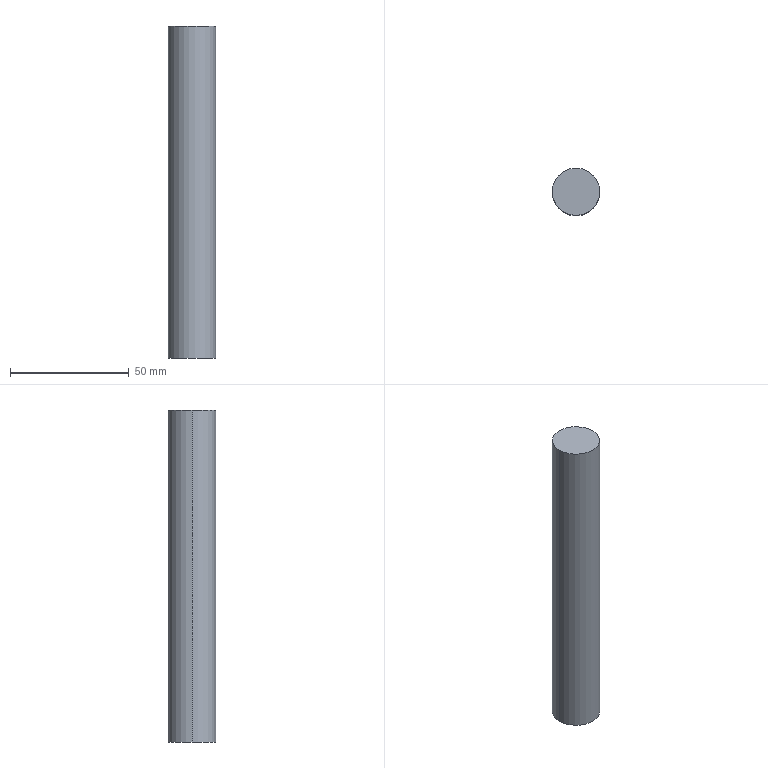Part | STEP file | 1 solid | 4 faces | box 20 x 20 x 140 mm | volume 43982 mm3 | cylinder 2 | plane 2 | commonest cylinder face diameters 20 x2
STEP:
#1=CARTESIAN_POINT('',(0.,0.,0.));
#2=DIRECTION('',(0.,0.,1.));
#3=DIRECTION('',(1.,0.,0.));
#4=AXIS2_PLACEMENT_3D('',#1,#2,#3);
#5=CARTESIAN_POINT('',(10.,1.493,0.));
#6=VERTEX_POINT('',#5);
#7=CARTESIAN_POINT('',(-10.,1.493,0.));
#8=VERTEX_POINT('',#7);
#9=CARTESIAN_POINT('',(0.,1.493,0.));
#10=DIRECTION('',(0.,0.,1.));
#11=DIRECTION('',(1.,0.,0.));
#12=AXIS2_PLACEMENT_3D('',#9,#10,#11);
#13=CIRCLE('',#12,10.);
#14=CARTESIAN_POINT('',(0.,1.493,0.));
#15=DIRECTION('',(0.,0.,1.));
#16=DIRECTION('',(1.,0.,0.));
#17=AXIS2_PLACEMENT_3D('',#14,#15,#16);
#18=CYLINDRICAL_SURFACE('',#17,10.);
#19=CARTESIAN_POINT('',(0.,0.));
#20=DIRECTION('',(1.,0.));
#21=VECTOR('',#20,1.);
#22=LINE('',#19,#21);
#23=(GEOMETRIC_REPRESENTATION_CONTEXT(2)PARAMETRIC_REPRESENTATION_CONTEXT()REPRESENTATION_CONTEXT('',''));
#24=DEFINITIONAL_REPRESENTATION('',(#22),#23);
#25=PCURVE('',#18,#24);
#26=CARTESIAN_POINT('',(0.,1.493,0.));
#27=DIRECTION('',(0.,0.,1.));
#28=DIRECTION('',(1.,0.,0.));
#29=AXIS2_PLACEMENT_3D('',#26,#27,#28);
#30=PLANE('',#29);
#31=CARTESIAN_POINT('',(0.,0.));
#32=DIRECTION('',(1.,0.));
#33=AXIS2_PLACEMENT_2D('',#31,#32);
#34=CIRCLE('',#33,10.);
#35=(GEOMETRIC_REPRESENTATION_CONTEXT(2)PARAMETRIC_REPRESENTATION_CONTEXT()REPRESENTATION_CONTEXT('',''));
#36=DEFINITIONAL_REPRESENTATION('',(#34),#35);
#37=PCURVE('',#30,#36);
#38=SURFACE_CURVE('',#13,(#25,#37),.PCURVE_S1.);
#39=EDGE_CURVE('',#6,#8,#38,.T.);
#40=ORIENTED_EDGE('',*,*,#39,.T.);
#41=CARTESIAN_POINT('',(-10.,1.493,140.));
#42=VERTEX_POINT('',#41);
#43=CARTESIAN_POINT('',(-10.,1.493,0.));
#44=DIRECTION('',(0.,0.,1.));
#45=VECTOR('',#44,1.);
#46=LINE('',#43,#45);
#47=CARTESIAN_POINT('',(3.142,0.));
#48=DIRECTION('',(0.,1.));
#49=VECTOR('',#48,1.);
#50=LINE('',#47,#49);
#51=(GEOMETRIC_REPRESENTATION_CONTEXT(2)PARAMETRIC_REPRESENTATION_CONTEXT()REPRESENTATION_CONTEXT('',''));
#52=DEFINITIONAL_REPRESENTATION('',(#50),#51);
#53=PCURVE('',#18,#52);
#54=CARTESIAN_POINT('',(0.,1.493,0.));
#55=DIRECTION('',(0.,0.,1.));
#56=DIRECTION('',(1.,0.,0.));
#57=AXIS2_PLACEMENT_3D('',#54,#55,#56);
#58=CYLINDRICAL_SURFACE('',#57,10.);
#59=CARTESIAN_POINT('',(3.142,0.));
#60=DIRECTION('',(0.,1.));
#61=VECTOR('',#60,1.);
#62=LINE('',#59,#61);
#63=(GEOMETRIC_REPRESENTATION_CONTEXT(2)PARAMETRIC_REPRESENTATION_CONTEXT()REPRESENTATION_CONTEXT('',''));
#64=DEFINITIONAL_REPRESENTATION('',(#62),#63);
#65=PCURVE('',#58,#64);
#66=SURFACE_CURVE('',#46,(#53,#65),.PCURVE_S1.);
#67=EDGE_CURVE('',#8,#42,#66,.T.);
#68=ORIENTED_EDGE('',*,*,#67,.T.);
#69=CARTESIAN_POINT('',(10.,1.493,140.));
#70=VERTEX_POINT('',#69);
#71=CARTESIAN_POINT('',(0.,1.493,140.));
#72=DIRECTION('',(0.,0.,-1.));
#73=DIRECTION('',(1.,0.,0.));
#74=AXIS2_PLACEMENT_3D('',#71,#72,#73);
#75=CIRCLE('',#74,10.);
#76=CARTESIAN_POINT('',(6.283,140.));
#77=DIRECTION('',(-1.,0.));
#78=VECTOR('',#77,1.);
#79=LINE('',#76,#78);
#80=(GEOMETRIC_REPRESENTATION_CONTEXT(2)PARAMETRIC_REPRESENTATION_CONTEXT()REPRESENTATION_CONTEXT('',''));
#81=DEFINITIONAL_REPRESENTATION('',(#79),#80);
#82=PCURVE('',#18,#81);
#83=CARTESIAN_POINT('',(0.,1.493,140.));
#84=DIRECTION('',(0.,0.,1.));
#85=DIRECTION('',(1.,0.,0.));
#86=AXIS2_PLACEMENT_3D('',#83,#84,#85);
#87=PLANE('',#86);
#88=CARTESIAN_POINT('',(10.,0.));
#89=CARTESIAN_POINT('',(10.,-17.321));
#90=CARTESIAN_POINT('',(-5.,-8.66));
#91=CARTESIAN_POINT('',(-20.,0.));
#92=CARTESIAN_POINT('',(-5.,8.66));
#93=CARTESIAN_POINT('',(10.,17.321));
#94=CARTESIAN_POINT('',(10.,0.));
#95=(BOUNDED_CURVE()B_SPLINE_CURVE(2,(#88,#89,#90,#91,#92,#93,#94),.UNSPECIFIED.,.T.,.F.)B_SPLINE_CURVE_WITH_KNOTS((1,2,2,2,2,1),(-2.094,0.,2.094,4.189,6.283,8.378),.UNSPECIFIED.)CURVE()GEOMETRIC_REPRESENTATION_ITEM()RATIONAL_B_SPLINE_CURVE((1.,0.5,1.,0.5,1.,0.5,1.))REPRESENTATION_ITEM(''));
#96=(GEOMETRIC_REPRESENTATION_CONTEXT(2)PARAMETRIC_REPRESENTATION_CONTEXT()REPRESENTATION_CONTEXT('',''));
#97=DEFINITIONAL_REPRESENTATION('',(#95),#96);
#98=PCURVE('',#87,#97);
#99=SURFACE_CURVE('',#75,(#82,#98),.PCURVE_S1.);
#100=EDGE_CURVE('',#42,#70,#99,.T.);
#101=ORIENTED_EDGE('',*,*,#100,.T.);
#102=CARTESIAN_POINT('',(10.,1.493,0.));
#103=DIRECTION('',(0.,0.,1.));
#104=VECTOR('',#103,1.);
#105=LINE('',#102,#104);
#106=CARTESIAN_POINT('',(0.,0.));
#107=DIRECTION('',(0.,1.));
#108=VECTOR('',#107,1.);
#109=LINE('',#106,#108);
#110=(GEOMETRIC_REPRESENTATION_CONTEXT(2)PARAMETRIC_REPRESENTATION_CONTEXT()REPRESENTATION_CONTEXT('',''));
#111=DEFINITIONAL_REPRESENTATION('',(#109),#110);
#112=PCURVE('',#18,#111);
#113=CARTESIAN_POINT('',(6.283,0.));
#114=DIRECTION('',(0.,1.));
#115=VECTOR('',#114,1.);
#116=LINE('',#113,#115);
#117=(GEOMETRIC_REPRESENTATION_CONTEXT(2)PARAMETRIC_REPRESENTATION_CONTEXT()REPRESENTATION_CONTEXT('',''));
#118=DEFINITIONAL_REPRESENTATION('',(#116),#117);
#119=PCURVE('',#58,#118);
#120=SURFACE_CURVE('',#105,(#112,#119),.PCURVE_S1.);
#121=EDGE_CURVE('',#6,#70,#120,.T.);
#122=ORIENTED_EDGE('',*,*,#121,.F.);
#123=EDGE_LOOP('',(#40,#68,#101,#122));
#124=FACE_BOUND('',#123,.T.);
#125=ADVANCED_FACE('',(#124),#18,.T.);
#126=ORIENTED_EDGE('',*,*,#67,.F.);
#127=CARTESIAN_POINT('',(0.,1.493,0.));
#128=DIRECTION('',(0.,0.,1.));
#129=DIRECTION('',(1.,0.,0.));
#130=AXIS2_PLACEMENT_3D('',#127,#128,#129);
#131=CIRCLE('',#130,10.);
#132=CARTESIAN_POINT('',(0.,0.));
#133=DIRECTION('',(1.,0.));
#134=VECTOR('',#133,1.);
#135=LINE('',#132,#134);
#136=(GEOMETRIC_REPRESENTATION_CONTEXT(2)PARAMETRIC_REPRESENTATION_CONTEXT()REPRESENTATION_CONTEXT('',''));
#137=DEFINITIONAL_REPRESENTATION('',(#135),#136);
#138=PCURVE('',#58,#137);
#139=CARTESIAN_POINT('',(0.,0.));
#140=DIRECTION('',(1.,0.));
#141=AXIS2_PLACEMENT_2D('',#139,#140);
#142=CIRCLE('',#141,10.);
#143=(GEOMETRIC_REPRESENTATION_CONTEXT(2)PARAMETRIC_REPRESENTATION_CONTEXT()REPRESENTATION_CONTEXT('',''));
#144=DEFINITIONAL_REPRESENTATION('',(#142),#143);
#145=PCURVE('',#30,#144);
#146=SURFACE_CURVE('',#131,(#138,#145),.PCURVE_S1.);
#147=EDGE_CURVE('',#8,#6,#146,.T.);
#148=ORIENTED_EDGE('',*,*,#147,.T.);
#149=ORIENTED_EDGE('',*,*,#121,.T.);
#150=CARTESIAN_POINT('',(0.,1.493,140.));
#151=DIRECTION('',(0.,0.,-1.));
#152=DIRECTION('',(1.,0.,0.));
#153=AXIS2_PLACEMENT_3D('',#150,#151,#152);
#154=CIRCLE('',#153,10.);
#155=CARTESIAN_POINT('',(6.283,140.));
#156=DIRECTION('',(-1.,0.));
#157=VECTOR('',#156,1.);
#158=LINE('',#155,#157);
#159=(GEOMETRIC_REPRESENTATION_CONTEXT(2)PARAMETRIC_REPRESENTATION_CONTEXT()REPRESENTATION_CONTEXT('',''));
#160=DEFINITIONAL_REPRESENTATION('',(#158),#159);
#161=PCURVE('',#58,#160);
#162=CARTESIAN_POINT('',(10.,0.));
#163=CARTESIAN_POINT('',(10.,-17.321));
#164=CARTESIAN_POINT('',(-5.,-8.66));
#165=CARTESIAN_POINT('',(-20.,0.));
#166=CARTESIAN_POINT('',(-5.,8.66));
#167=CARTESIAN_POINT('',(10.,17.321));
#168=CARTESIAN_POINT('',(10.,0.));
#169=(BOUNDED_CURVE()B_SPLINE_CURVE(2,(#162,#163,#164,#165,#166,#167,#168),.UNSPECIFIED.,.T.,.F.)B_SPLINE_CURVE_WITH_KNOTS((1,2,2,2,2,1),(-2.094,0.,2.094,4.189,6.283,8.378),.UNSPECIFIED.)CURVE()GEOMETRIC_REPRESENTATION_ITEM()RATIONAL_B_SPLINE_CURVE((1.,0.5,1.,0.5,1.,0.5,1.))REPRESENTATION_ITEM(''));
#170=(GEOMETRIC_REPRESENTATION_CONTEXT(2)PARAMETRIC_REPRESENTATION_CONTEXT()REPRESENTATION_CONTEXT('',''));
#171=DEFINITIONAL_REPRESENTATION('',(#169),#170);
#172=PCURVE('',#87,#171);
#173=SURFACE_CURVE('',#154,(#161,#172),.PCURVE_S1.);
#174=EDGE_CURVE('',#70,#42,#173,.T.);
#175=ORIENTED_EDGE('',*,*,#174,.T.);
#176=EDGE_LOOP('',(#126,#148,#149,#175));
#177=FACE_BOUND('',#176,.T.);
#178=ADVANCED_FACE('',(#177),#58,.T.);
#179=ORIENTED_EDGE('',*,*,#39,.F.);
#180=ORIENTED_EDGE('',*,*,#147,.F.);
#181=EDGE_LOOP('',(#179,#180));
#182=FACE_BOUND('',#181,.T.);
#183=ADVANCED_FACE('',(#182),#30,.F.);
#184=ORIENTED_EDGE('',*,*,#174,.F.);
#185=ORIENTED_EDGE('',*,*,#100,.F.);
#186=EDGE_LOOP('',(#184,#185));
#187=FACE_BOUND('',#186,.T.);
#188=ADVANCED_FACE('',(#187),#87,.T.);
#189=CLOSED_SHELL('',(#125,#178,#183,#188));
#190=MANIFOLD_SOLID_BREP('',#189);
#191=(LENGTH_UNIT()NAMED_UNIT(*)SI_UNIT(.MILLI.,.METRE.));
#192=UNCERTAINTY_MEASURE_WITH_UNIT(LENGTH_MEASURE(0.0000001),#191,'','');
#193=(NAMED_UNIT(*)PLANE_ANGLE_UNIT()SI_UNIT($,.RADIAN.));
#194=(NAMED_UNIT(*)SI_UNIT($,.STERADIAN.)SOLID_ANGLE_UNIT());
#195=(GEOMETRIC_REPRESENTATION_CONTEXT(3)GLOBAL_UNCERTAINTY_ASSIGNED_CONTEXT((#192))GLOBAL_UNIT_ASSIGNED_CONTEXT((#191,#193,#194))REPRESENTATION_CONTEXT('',''));
#196=ADVANCED_BREP_SHAPE_REPRESENTATION('',(#4,#190),#195);